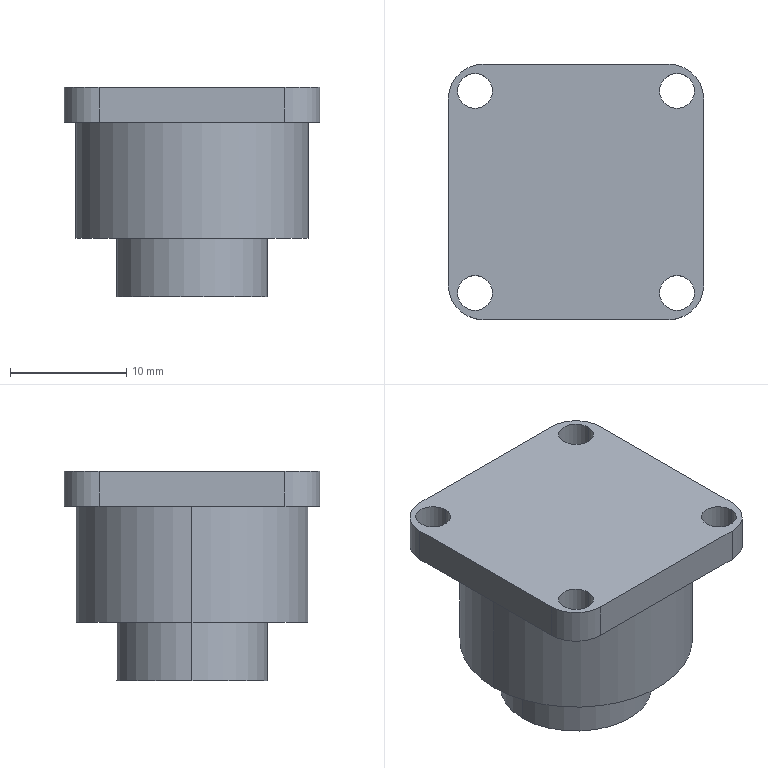Part | SolidWorks | features ICE 2, Cut 1, Extrusion 1, Fillet 1 | 1 solid | 27 faces | box 22 x 22 x 18 mm | volume 5008 mm3 | cylinder 18 | plane 9 | commonest cylinder face diameters 3 x8 6 x6 13 x2 20 x2
STEP:
#1=CARTESIAN_POINT('',(-155.946,-8.7,18.));
#2=VERTEX_POINT('',#1);
#3=CARTESIAN_POINT('',(-158.946,-8.7,18.));
#4=VERTEX_POINT('',#3);
#5=CARTESIAN_POINT('',(-157.446,-8.7,18.));
#6=DIRECTION('',(0.,0.,-1.));
#7=DIRECTION('',(-1.,0.,0.));
#8=AXIS2_PLACEMENT_3D('',#5,#6,#7);
#9=CIRCLE('',#8,1.5);
#10=EDGE_CURVE('',#2,#4,#9,.T.);
#11=ORIENTED_EDGE('',*,*,#10,.F.);
#12=CARTESIAN_POINT('',(-155.946,-8.7,15.));
#13=VERTEX_POINT('',#12);
#14=CARTESIAN_POINT('',(-155.946,-8.7,18.));
#15=DIRECTION('',(0.,0.,-1.));
#16=VECTOR('',#15,1000.);
#17=LINE('',#14,#16);
#18=EDGE_CURVE('',#2,#13,#17,.T.);
#19=ORIENTED_EDGE('',*,*,#18,.T.);
#20=CARTESIAN_POINT('',(-158.946,-8.7,15.));
#21=VERTEX_POINT('',#20);
#22=CARTESIAN_POINT('',(-157.446,-8.7,15.));
#23=DIRECTION('',(0.,0.,-1.));
#24=DIRECTION('',(-1.,0.,0.));
#25=AXIS2_PLACEMENT_3D('',#22,#23,#24);
#26=CIRCLE('',#25,1.5);
#27=EDGE_CURVE('',#13,#21,#26,.T.);
#28=ORIENTED_EDGE('',*,*,#27,.T.);
#29=CARTESIAN_POINT('',(-158.946,-8.7,18.));
#30=DIRECTION('',(0.,0.,-1.));
#31=VECTOR('',#30,1000.);
#32=LINE('',#29,#31);
#33=EDGE_CURVE('',#4,#21,#32,.T.);
#34=ORIENTED_EDGE('',*,*,#33,.F.);
#35=EDGE_LOOP('',(#11,#19,#28,#34));
#36=FACE_OUTER_BOUND('',#35,.T.);
#37=CARTESIAN_POINT('',(-157.446,-8.7,18.));
#38=DIRECTION('',(0.,0.,-1.));
#39=DIRECTION('',(-1.,0.,0.));
#40=AXIS2_PLACEMENT_3D('',#37,#38,#39);
#41=CYLINDRICAL_SURFACE('',#40,1.5);
#42=ADVANCED_FACE('',(#36),#41,.F.);
#43=CARTESIAN_POINT('',(-138.546,-8.7,18.));
#44=VERTEX_POINT('',#43);
#45=CARTESIAN_POINT('',(-141.546,-8.7,18.));
#46=VERTEX_POINT('',#45);
#47=CARTESIAN_POINT('',(-140.046,-8.7,18.));
#48=DIRECTION('',(0.,0.,-1.));
#49=DIRECTION('',(-1.,0.,0.));
#50=AXIS2_PLACEMENT_3D('',#47,#48,#49);
#51=CIRCLE('',#50,1.5);
#52=EDGE_CURVE('',#44,#46,#51,.T.);
#53=ORIENTED_EDGE('',*,*,#52,.F.);
#54=CARTESIAN_POINT('',(-138.546,-8.7,15.));
#55=VERTEX_POINT('',#54);
#56=CARTESIAN_POINT('',(-138.546,-8.7,18.));
#57=DIRECTION('',(0.,0.,-1.));
#58=VECTOR('',#57,1000.);
#59=LINE('',#56,#58);
#60=EDGE_CURVE('',#44,#55,#59,.T.);
#61=ORIENTED_EDGE('',*,*,#60,.T.);
#62=CARTESIAN_POINT('',(-141.546,-8.7,15.));
#63=VERTEX_POINT('',#62);
#64=CARTESIAN_POINT('',(-140.046,-8.7,15.));
#65=DIRECTION('',(0.,0.,-1.));
#66=DIRECTION('',(-1.,0.,0.));
#67=AXIS2_PLACEMENT_3D('',#64,#65,#66);
#68=CIRCLE('',#67,1.5);
#69=EDGE_CURVE('',#55,#63,#68,.T.);
#70=ORIENTED_EDGE('',*,*,#69,.T.);
#71=CARTESIAN_POINT('',(-141.546,-8.7,18.));
#72=DIRECTION('',(0.,0.,-1.));
#73=VECTOR('',#72,1000.);
#74=LINE('',#71,#73);
#75=EDGE_CURVE('',#46,#63,#74,.T.);
#76=ORIENTED_EDGE('',*,*,#75,.F.);
#77=EDGE_LOOP('',(#53,#61,#70,#76));
#78=FACE_OUTER_BOUND('',#77,.T.);
#79=CARTESIAN_POINT('',(-140.046,-8.7,18.));
#80=DIRECTION('',(0.,0.,-1.));
#81=DIRECTION('',(-1.,0.,0.));
#82=AXIS2_PLACEMENT_3D('',#79,#80,#81);
#83=CYLINDRICAL_SURFACE('',#82,1.5);
#84=ADVANCED_FACE('',(#78),#83,.F.);
#85=CARTESIAN_POINT('',(-138.546,8.7,18.));
#86=VERTEX_POINT('',#85);
#87=CARTESIAN_POINT('',(-141.546,8.7,18.));
#88=VERTEX_POINT('',#87);
#89=CARTESIAN_POINT('',(-140.046,8.7,18.));
#90=DIRECTION('',(0.,0.,-1.));
#91=DIRECTION('',(-1.,0.,0.));
#92=AXIS2_PLACEMENT_3D('',#89,#90,#91);
#93=CIRCLE('',#92,1.5);
#94=EDGE_CURVE('',#86,#88,#93,.T.);
#95=ORIENTED_EDGE('',*,*,#94,.F.);
#96=CARTESIAN_POINT('',(-138.546,8.7,15.));
#97=VERTEX_POINT('',#96);
#98=CARTESIAN_POINT('',(-138.546,8.7,18.));
#99=DIRECTION('',(0.,0.,-1.));
#100=VECTOR('',#99,1000.);
#101=LINE('',#98,#100);
#102=EDGE_CURVE('',#86,#97,#101,.T.);
#103=ORIENTED_EDGE('',*,*,#102,.T.);
#104=CARTESIAN_POINT('',(-141.546,8.7,15.));
#105=VERTEX_POINT('',#104);
#106=CARTESIAN_POINT('',(-140.046,8.7,15.));
#107=DIRECTION('',(0.,0.,-1.));
#108=DIRECTION('',(-1.,0.,0.));
#109=AXIS2_PLACEMENT_3D('',#106,#107,#108);
#110=CIRCLE('',#109,1.5);
#111=EDGE_CURVE('',#97,#105,#110,.T.);
#112=ORIENTED_EDGE('',*,*,#111,.T.);
#113=CARTESIAN_POINT('',(-141.546,8.7,18.));
#114=DIRECTION('',(0.,0.,-1.));
#115=VECTOR('',#114,1000.);
#116=LINE('',#113,#115);
#117=EDGE_CURVE('',#88,#105,#116,.T.);
#118=ORIENTED_EDGE('',*,*,#117,.F.);
#119=EDGE_LOOP('',(#95,#103,#112,#118));
#120=FACE_OUTER_BOUND('',#119,.T.);
#121=CARTESIAN_POINT('',(-140.046,8.7,18.));
#122=DIRECTION('',(0.,0.,-1.));
#123=DIRECTION('',(-1.,0.,0.));
#124=AXIS2_PLACEMENT_3D('',#121,#122,#123);
#125=CYLINDRICAL_SURFACE('',#124,1.5);
#126=ADVANCED_FACE('',(#120),#125,.F.);
#127=CARTESIAN_POINT('',(-155.946,8.7,18.));
#128=VERTEX_POINT('',#127);
#129=CARTESIAN_POINT('',(-158.946,8.7,18.));
#130=VERTEX_POINT('',#129);
#131=CARTESIAN_POINT('',(-157.446,8.7,18.));
#132=DIRECTION('',(0.,0.,-1.));
#133=DIRECTION('',(-1.,0.,0.));
#134=AXIS2_PLACEMENT_3D('',#131,#132,#133);
#135=CIRCLE('',#134,1.5);
#136=EDGE_CURVE('',#128,#130,#135,.T.);
#137=ORIENTED_EDGE('',*,*,#136,.F.);
#138=CARTESIAN_POINT('',(-155.946,8.7,15.));
#139=VERTEX_POINT('',#138);
#140=CARTESIAN_POINT('',(-155.946,8.7,18.));
#141=DIRECTION('',(0.,0.,-1.));
#142=VECTOR('',#141,1000.);
#143=LINE('',#140,#142);
#144=EDGE_CURVE('',#128,#139,#143,.T.);
#145=ORIENTED_EDGE('',*,*,#144,.T.);
#146=CARTESIAN_POINT('',(-158.946,8.7,15.));
#147=VERTEX_POINT('',#146);
#148=CARTESIAN_POINT('',(-157.446,8.7,15.));
#149=DIRECTION('',(0.,0.,-1.));
#150=DIRECTION('',(-1.,0.,0.));
#151=AXIS2_PLACEMENT_3D('',#148,#149,#150);
#152=CIRCLE('',#151,1.5);
#153=EDGE_CURVE('',#139,#147,#152,.T.);
#154=ORIENTED_EDGE('',*,*,#153,.T.);
#155=CARTESIAN_POINT('',(-158.946,8.7,18.));
#156=DIRECTION('',(0.,0.,-1.));
#157=VECTOR('',#156,1000.);
#158=LINE('',#155,#157);
#159=EDGE_CURVE('',#130,#147,#158,.T.);
#160=ORIENTED_EDGE('',*,*,#159,.F.);
#161=EDGE_LOOP('',(#137,#145,#154,#160));
#162=FACE_OUTER_BOUND('',#161,.T.);
#163=CARTESIAN_POINT('',(-157.446,8.7,18.));
#164=DIRECTION('',(0.,0.,-1.));
#165=DIRECTION('',(-1.,0.,0.));
#166=AXIS2_PLACEMENT_3D('',#163,#164,#165);
#167=CYLINDRICAL_SURFACE('',#166,1.5);
#168=ADVANCED_FACE('',(#162),#167,.F.);
#169=CARTESIAN_POINT('',(-138.746,0.,15.));
#170=VERTEX_POINT('',#169);
#171=CARTESIAN_POINT('',(-158.746,0.,15.));
#172=VERTEX_POINT('',#171);
#173=CARTESIAN_POINT('',(-148.746,0.,15.));
#174=DIRECTION('',(0.,0.,1.));
#175=DIRECTION('',(1.,0.,0.));
#176=AXIS2_PLACEMENT_3D('',#173,#174,#175);
#177=CIRCLE('',#176,10.);
#178=EDGE_CURVE('',#170,#172,#177,.T.);
#179=ORIENTED_EDGE('',*,*,#178,.F.);
#180=CARTESIAN_POINT('',(-138.746,0.,5.));
#181=VERTEX_POINT('',#180);
#182=CARTESIAN_POINT('',(-138.746,0.,15.));
#183=DIRECTION('',(0.,0.,-1.));
#184=VECTOR('',#183,1000.);
#185=LINE('',#182,#184);
#186=EDGE_CURVE('',#170,#181,#185,.T.);
#187=ORIENTED_EDGE('',*,*,#186,.T.);
#188=CARTESIAN_POINT('',(-158.746,0.,5.));
#189=VERTEX_POINT('',#188);
#190=CARTESIAN_POINT('',(-148.746,0.,5.));
#191=DIRECTION('',(0.,0.,1.));
#192=DIRECTION('',(1.,0.,0.));
#193=AXIS2_PLACEMENT_3D('',#190,#191,#192);
#194=CIRCLE('',#193,10.);
#195=EDGE_CURVE('',#181,#189,#194,.T.);
#196=ORIENTED_EDGE('',*,*,#195,.T.);
#197=CARTESIAN_POINT('',(-158.746,0.,15.));
#198=DIRECTION('',(0.,0.,-1.));
#199=VECTOR('',#198,1000.);
#200=LINE('',#197,#199);
#201=EDGE_CURVE('',#172,#189,#200,.T.);
#202=ORIENTED_EDGE('',*,*,#201,.F.);
#203=EDGE_LOOP('',(#179,#187,#196,#202));
#204=FACE_OUTER_BOUND('',#203,.T.);
#205=CARTESIAN_POINT('',(-148.746,0.,15.));
#206=DIRECTION('',(0.,0.,-1.));
#207=DIRECTION('',(-1.,0.,0.));
#208=AXIS2_PLACEMENT_3D('',#205,#206,#207);
#209=CYLINDRICAL_SURFACE('',#208,10.);
#210=ADVANCED_FACE('',(#204),#209,.T.);
#211=CARTESIAN_POINT('',(-151.746,0.,5.));
#212=VERTEX_POINT('',#211);
#213=CARTESIAN_POINT('',(-145.746,0.,5.));
#214=VERTEX_POINT('',#213);
#215=CARTESIAN_POINT('',(-148.746,0.,5.));
#216=DIRECTION('',(0.,0.,1.));
#217=DIRECTION('',(1.,0.,0.));
#218=AXIS2_PLACEMENT_3D('',#215,#216,#217);
#219=CIRCLE('',#218,3.);
#220=EDGE_CURVE('',#212,#214,#219,.T.);
#221=ORIENTED_EDGE('',*,*,#220,.T.);
#222=CARTESIAN_POINT('',(-145.746,0.,0.));
#223=VERTEX_POINT('',#222);
#224=CARTESIAN_POINT('',(-145.746,0.,5.));
#225=DIRECTION('',(0.,0.,-1.));
#226=VECTOR('',#225,1000.);
#227=LINE('',#224,#226);
#228=EDGE_CURVE('',#214,#223,#227,.T.);
#229=ORIENTED_EDGE('',*,*,#228,.T.);
#230=CARTESIAN_POINT('',(-151.746,0.,0.));
#231=VERTEX_POINT('',#230);
#232=CARTESIAN_POINT('',(-148.746,0.,0.));
#233=DIRECTION('',(0.,0.,1.));
#234=DIRECTION('',(1.,0.,0.));
#235=AXIS2_PLACEMENT_3D('',#232,#233,#234);
#236=CIRCLE('',#235,3.);
#237=EDGE_CURVE('',#231,#223,#236,.T.);
#238=ORIENTED_EDGE('',*,*,#237,.F.);
#239=CARTESIAN_POINT('',(-151.746,0.,5.));
#240=DIRECTION('',(0.,0.,-1.));
#241=VECTOR('',#240,1000.);
#242=LINE('',#239,#241);
#243=EDGE_CURVE('',#212,#231,#242,.T.);
#244=ORIENTED_EDGE('',*,*,#243,.F.);
#245=EDGE_LOOP('',(#221,#229,#238,#244));
#246=FACE_OUTER_BOUND('',#245,.T.);
#247=CARTESIAN_POINT('',(-148.746,0.,5.));
#248=DIRECTION('',(0.,0.,-1.));
#249=DIRECTION('',(-1.,0.,0.));
#250=AXIS2_PLACEMENT_3D('',#247,#248,#249);
#251=CYLINDRICAL_SURFACE('',#250,3.);
#252=ADVANCED_FACE('',(#246),#251,.F.);
#253=CARTESIAN_POINT('',(-142.246,0.,5.));
#254=VERTEX_POINT('',#253);
#255=CARTESIAN_POINT('',(-155.246,0.,5.));
#256=VERTEX_POINT('',#255);
#257=CARTESIAN_POINT('',(-148.746,0.,5.));
#258=DIRECTION('',(0.,0.,1.));
#259=DIRECTION('',(1.,0.,0.));
#260=AXIS2_PLACEMENT_3D('',#257,#258,#259);
#261=CIRCLE('',#260,6.5);
#262=EDGE_CURVE('',#254,#256,#261,.T.);
#263=ORIENTED_EDGE('',*,*,#262,.F.);
#264=CARTESIAN_POINT('',(-142.246,0.,0.));
#265=VERTEX_POINT('',#264);
#266=CARTESIAN_POINT('',(-142.246,0.,5.));
#267=DIRECTION('',(0.,0.,-1.));
#268=VECTOR('',#267,1000.);
#269=LINE('',#266,#268);
#270=EDGE_CURVE('',#254,#265,#269,.T.);
#271=ORIENTED_EDGE('',*,*,#270,.T.);
#272=CARTESIAN_POINT('',(-155.246,0.,0.));
#273=VERTEX_POINT('',#272);
#274=CARTESIAN_POINT('',(-148.746,0.,0.));
#275=DIRECTION('',(0.,0.,1.));
#276=DIRECTION('',(1.,0.,0.));
#277=AXIS2_PLACEMENT_3D('',#274,#275,#276);
#278=CIRCLE('',#277,6.5);
#279=EDGE_CURVE('',#265,#273,#278,.T.);
#280=ORIENTED_EDGE('',*,*,#279,.T.);
#281=CARTESIAN_POINT('',(-155.246,0.,5.));
#282=DIRECTION('',(0.,0.,-1.));
#283=VECTOR('',#282,1000.);
#284=LINE('',#281,#283);
#285=EDGE_CURVE('',#256,#273,#284,.T.);
#286=ORIENTED_EDGE('',*,*,#285,.F.);
#287=EDGE_LOOP('',(#263,#271,#280,#286));
#288=FACE_OUTER_BOUND('',#287,.T.);
#289=CARTESIAN_POINT('',(-148.746,0.,5.));
#290=DIRECTION('',(0.,0.,-1.));
#291=DIRECTION('',(-1.,0.,0.));
#292=AXIS2_PLACEMENT_3D('',#289,#290,#291);
#293=CYLINDRICAL_SURFACE('',#292,6.5);
#294=ADVANCED_FACE('',(#288),#293,.T.);
#295=CARTESIAN_POINT('',(-148.746,0.,0.));
#296=DIRECTION('',(0.,0.,1.));
#297=DIRECTION('',(1.,0.,0.));
#298=AXIS2_PLACEMENT_3D('',#295,#296,#297);
#299=CIRCLE('',#298,6.5);
#300=EDGE_CURVE('',#273,#265,#299,.T.);
#301=ORIENTED_EDGE('',*,*,#300,.F.);
#302=ORIENTED_EDGE('',*,*,#279,.F.);
#303=EDGE_LOOP('',(#301,#302));
#304=FACE_OUTER_BOUND('',#303,.T.);
#305=ORIENTED_EDGE('',*,*,#237,.T.);
#306=CARTESIAN_POINT('',(-148.746,0.,0.));
#307=DIRECTION('',(0.,0.,1.));
#308=DIRECTION('',(1.,0.,0.));
#309=AXIS2_PLACEMENT_3D('',#306,#307,#308);
#310=CIRCLE('',#309,3.);
#311=EDGE_CURVE('',#223,#231,#310,.T.);
#312=ORIENTED_EDGE('',*,*,#311,.T.);
#313=EDGE_LOOP('',(#305,#312));
#314=FACE_BOUND('',#313,.T.);
#315=CARTESIAN_POINT('',(-148.746,0.,0.));
#316=DIRECTION('',(0.,0.,1.));
#317=DIRECTION('',(1.,0.,0.));
#318=AXIS2_PLACEMENT_3D('',#315,#316,#317);
#319=PLANE('',#318);
#320=ADVANCED_FACE('',(#304,#314),#319,.F.);
#321=ORIENTED_EDGE('',*,*,#270,.F.);
#322=CARTESIAN_POINT('',(-148.746,0.,5.));
#323=DIRECTION('',(0.,0.,1.));
#324=DIRECTION('',(1.,0.,0.));
#325=AXIS2_PLACEMENT_3D('',#322,#323,#324);
#326=CIRCLE('',#325,6.5);
#327=EDGE_CURVE('',#256,#254,#326,.T.);
#328=ORIENTED_EDGE('',*,*,#327,.F.);
#329=ORIENTED_EDGE('',*,*,#285,.T.);
#330=ORIENTED_EDGE('',*,*,#300,.T.);
#331=EDGE_LOOP('',(#321,#328,#329,#330));
#332=FACE_OUTER_BOUND('',#331,.T.);
#333=CARTESIAN_POINT('',(-148.746,0.,5.));
#334=DIRECTION('',(0.,0.,-1.));
#335=DIRECTION('',(-1.,0.,0.));
#336=AXIS2_PLACEMENT_3D('',#333,#334,#335);
#337=CYLINDRICAL_SURFACE('',#336,6.5);
#338=ADVANCED_FACE('',(#332),#337,.T.);
#339=ORIENTED_EDGE('',*,*,#228,.F.);
#340=CARTESIAN_POINT('',(-148.746,0.,5.));
#341=DIRECTION('',(0.,0.,1.));
#342=DIRECTION('',(1.,0.,0.));
#343=AXIS2_PLACEMENT_3D('',#340,#341,#342);
#344=CIRCLE('',#343,3.);
#345=EDGE_CURVE('',#214,#212,#344,.T.);
#346=ORIENTED_EDGE('',*,*,#345,.T.);
#347=ORIENTED_EDGE('',*,*,#243,.T.);
#348=ORIENTED_EDGE('',*,*,#311,.F.);
#349=EDGE_LOOP('',(#339,#346,#347,#348));
#350=FACE_OUTER_BOUND('',#349,.T.);
#351=CARTESIAN_POINT('',(-148.746,0.,5.));
#352=DIRECTION('',(0.,0.,-1.));
#353=DIRECTION('',(-1.,0.,0.));
#354=AXIS2_PLACEMENT_3D('',#351,#352,#353);
#355=CYLINDRICAL_SURFACE('',#354,3.);
#356=ADVANCED_FACE('',(#350),#355,.F.);
#357=ORIENTED_EDGE('',*,*,#220,.F.);
#358=ORIENTED_EDGE('',*,*,#345,.F.);
#359=EDGE_LOOP('',(#357,#358));
#360=FACE_OUTER_BOUND('',#359,.T.);
#361=CARTESIAN_POINT('',(-148.746,0.,5.));
#362=DIRECTION('',(0.,0.,1.));
#363=DIRECTION('',(1.,0.,0.));
#364=AXIS2_PLACEMENT_3D('',#361,#362,#363);
#365=PLANE('',#364);
#366=ADVANCED_FACE('',(#360),#365,.F.);
#367=ORIENTED_EDGE('',*,*,#186,.F.);
#368=CARTESIAN_POINT('',(-148.746,0.,15.));
#369=DIRECTION('',(0.,0.,1.));
#370=DIRECTION('',(1.,0.,0.));
#371=AXIS2_PLACEMENT_3D('',#368,#369,#370);
#372=CIRCLE('',#371,10.);
#373=EDGE_CURVE('',#172,#170,#372,.T.);
#374=ORIENTED_EDGE('',*,*,#373,.F.);
#375=ORIENTED_EDGE('',*,*,#201,.T.);
#376=CARTESIAN_POINT('',(-148.746,0.,5.));
#377=DIRECTION('',(0.,0.,1.));
#378=DIRECTION('',(1.,0.,0.));
#379=AXIS2_PLACEMENT_3D('',#376,#377,#378);
#380=CIRCLE('',#379,10.);
#381=EDGE_CURVE('',#189,#181,#380,.T.);
#382=ORIENTED_EDGE('',*,*,#381,.T.);
#383=EDGE_LOOP('',(#367,#374,#375,#382));
#384=FACE_OUTER_BOUND('',#383,.T.);
#385=CARTESIAN_POINT('',(-148.746,0.,15.));
#386=DIRECTION('',(0.,0.,-1.));
#387=DIRECTION('',(-1.,0.,0.));
#388=AXIS2_PLACEMENT_3D('',#385,#386,#387);
#389=CYLINDRICAL_SURFACE('',#388,10.);
#390=ADVANCED_FACE('',(#384),#389,.T.);
#391=ORIENTED_EDGE('',*,*,#327,.T.);
#392=ORIENTED_EDGE('',*,*,#262,.T.);
#393=EDGE_LOOP('',(#391,#392));
#394=FACE_BOUND('',#393,.T.);
#395=ORIENTED_EDGE('',*,*,#381,.F.);
#396=ORIENTED_EDGE('',*,*,#195,.F.);
#397=EDGE_LOOP('',(#395,#396));
#398=FACE_OUTER_BOUND('',#397,.T.);
#399=CARTESIAN_POINT('',(-148.746,0.,5.));
#400=DIRECTION('',(0.,0.,1.));
#401=DIRECTION('',(1.,0.,0.));
#402=AXIS2_PLACEMENT_3D('',#399,#400,#401);
#403=PLANE('',#402);
#404=ADVANCED_FACE('',(#394,#398),#403,.F.);
#405=CARTESIAN_POINT('',(-137.746,-8.,15.));
#406=VERTEX_POINT('',#405);
#407=CARTESIAN_POINT('',(-137.746,8.,15.));
#408=VERTEX_POINT('',#407);
#409=CARTESIAN_POINT('',(-137.746,-11.,15.));
#410=DIRECTION('',(0.,1.,0.));
#411=VECTOR('',#410,1000.);
#412=LINE('',#409,#411);
#413=EDGE_CURVE('',#406,#408,#412,.T.);
#414=ORIENTED_EDGE('',*,*,#413,.T.);
#415=CARTESIAN_POINT('',(-137.746,8.,18.));
#416=VERTEX_POINT('',#415);
#417=CARTESIAN_POINT('',(-137.746,8.,18.));
#418=DIRECTION('',(0.,0.,1.));
#419=VECTOR('',#418,1000.);
#420=LINE('',#417,#419);
#421=EDGE_CURVE('',#408,#416,#420,.T.);
#422=ORIENTED_EDGE('',*,*,#421,.T.);
#423=CARTESIAN_POINT('',(-137.746,-8.,18.));
#424=VERTEX_POINT('',#423);
#425=CARTESIAN_POINT('',(-137.746,-11.,18.));
#426=DIRECTION('',(0.,1.,0.));
#427=VECTOR('',#426,1000.);
#428=LINE('',#425,#427);
#429=EDGE_CURVE('',#424,#416,#428,.T.);
#430=ORIENTED_EDGE('',*,*,#429,.F.);
#431=CARTESIAN_POINT('',(-137.746,-8.,18.));
#432=DIRECTION('',(0.,0.,-1.));
#433=VECTOR('',#432,1000.);
#434=LINE('',#431,#433);
#435=EDGE_CURVE('',#424,#406,#434,.T.);
#436=ORIENTED_EDGE('',*,*,#435,.T.);
#437=EDGE_LOOP('',(#414,#422,#430,#436));
#438=FACE_OUTER_BOUND('',#437,.T.);
#439=CARTESIAN_POINT('',(-137.746,-11.,18.));
#440=DIRECTION('',(-1.,0.,0.));
#441=DIRECTION('',(0.,0.,1.));
#442=AXIS2_PLACEMENT_3D('',#439,#440,#441);
#443=PLANE('',#442);
#444=ADVANCED_FACE('',(#438),#443,.F.);
#445=CARTESIAN_POINT('',(-140.746,11.,18.));
#446=VERTEX_POINT('',#445);
#447=CARTESIAN_POINT('',(-156.746,11.,18.));
#448=VERTEX_POINT('',#447);
#449=CARTESIAN_POINT('',(-159.746,11.,18.));
#450=DIRECTION('',(-1.,0.,0.));
#451=VECTOR('',#450,1000.);
#452=LINE('',#449,#451);
#453=EDGE_CURVE('',#446,#448,#452,.T.);
#454=ORIENTED_EDGE('',*,*,#453,.F.);
#455=CARTESIAN_POINT('',(-140.746,11.,15.));
#456=VERTEX_POINT('',#455);
#457=CARTESIAN_POINT('',(-140.746,11.,18.));
#458=DIRECTION('',(0.,0.,-1.));
#459=VECTOR('',#458,1000.);
#460=LINE('',#457,#459);
#461=EDGE_CURVE('',#446,#456,#460,.T.);
#462=ORIENTED_EDGE('',*,*,#461,.T.);
#463=CARTESIAN_POINT('',(-156.746,11.,15.));
#464=VERTEX_POINT('',#463);
#465=CARTESIAN_POINT('',(-159.746,11.,15.));
#466=DIRECTION('',(-1.,0.,0.));
#467=VECTOR('',#466,1000.);
#468=LINE('',#465,#467);
#469=EDGE_CURVE('',#456,#464,#468,.T.);
#470=ORIENTED_EDGE('',*,*,#469,.T.);
#471=CARTESIAN_POINT('',(-156.746,11.,18.));
#472=DIRECTION('',(0.,0.,1.));
#473=VECTOR('',#472,1000.);
#474=LINE('',#471,#473);
#475=EDGE_CURVE('',#464,#448,#474,.T.);
#476=ORIENTED_EDGE('',*,*,#475,.T.);
#477=EDGE_LOOP('',(#454,#462,#470,#476));
#478=FACE_OUTER_BOUND('',#477,.T.);
#479=CARTESIAN_POINT('',(-159.746,11.,18.));
#480=DIRECTION('',(0.,-1.,0.));
#481=DIRECTION('',(0.,0.,-1.));
#482=AXIS2_PLACEMENT_3D('',#479,#480,#481);
#483=PLANE('',#482);
#484=ADVANCED_FACE('',(#478),#483,.F.);
#485=CARTESIAN_POINT('',(-159.746,8.,15.));
#486=VERTEX_POINT('',#485);
#487=CARTESIAN_POINT('',(-159.746,-8.,15.));
#488=VERTEX_POINT('',#487);
#489=CARTESIAN_POINT('',(-159.746,-11.,15.));
#490=DIRECTION('',(0.,-1.,0.));
#491=VECTOR('',#490,1000.);
#492=LINE('',#489,#491);
#493=EDGE_CURVE('',#486,#488,#492,.T.);
#494=ORIENTED_EDGE('',*,*,#493,.T.);
#495=CARTESIAN_POINT('',(-159.746,-8.,18.));
#496=VERTEX_POINT('',#495);
#497=CARTESIAN_POINT('',(-159.746,-8.,18.));
#498=DIRECTION('',(0.,0.,1.));
#499=VECTOR('',#498,1000.);
#500=LINE('',#497,#499);
#501=EDGE_CURVE('',#488,#496,#500,.T.);
#502=ORIENTED_EDGE('',*,*,#501,.T.);
#503=CARTESIAN_POINT('',(-159.746,8.,18.));
#504=VERTEX_POINT('',#503);
#505=CARTESIAN_POINT('',(-159.746,-11.,18.));
#506=DIRECTION('',(0.,-1.,0.));
#507=VECTOR('',#506,1000.);
#508=LINE('',#505,#507);
#509=EDGE_CURVE('',#504,#496,#508,.T.);
#510=ORIENTED_EDGE('',*,*,#509,.F.);
#511=CARTESIAN_POINT('',(-159.746,8.,18.));
#512=DIRECTION('',(0.,0.,-1.));
#513=VECTOR('',#512,1000.);
#514=LINE('',#511,#513);
#515=EDGE_CURVE('',#504,#486,#514,.T.);
#516=ORIENTED_EDGE('',*,*,#515,.T.);
#517=EDGE_LOOP('',(#494,#502,#510,#516));
#518=FACE_OUTER_BOUND('',#517,.T.);
#519=CARTESIAN_POINT('',(-159.746,-11.,18.));
#520=DIRECTION('',(1.,0.,0.));
#521=DIRECTION('',(0.,0.,-1.));
#522=AXIS2_PLACEMENT_3D('',#519,#520,#521);
#523=PLANE('',#522);
#524=ADVANCED_FACE('',(#518),#523,.F.);
#525=CARTESIAN_POINT('',(-156.746,-11.,18.));
#526=VERTEX_POINT('',#525);
#527=CARTESIAN_POINT('',(-140.746,-11.,18.));
#528=VERTEX_POINT('',#527);
#529=CARTESIAN_POINT('',(-159.746,-11.,18.));
#530=DIRECTION('',(1.,0.,0.));
#531=VECTOR('',#530,1000.);
#532=LINE('',#529,#531);
#533=EDGE_CURVE('',#526,#528,#532,.T.);
#534=ORIENTED_EDGE('',*,*,#533,.F.);
#535=CARTESIAN_POINT('',(-156.746,-11.,15.));
#536=VERTEX_POINT('',#535);
#537=CARTESIAN_POINT('',(-156.746,-11.,18.));
#538=DIRECTION('',(0.,0.,-1.));
#539=VECTOR('',#538,1000.);
#540=LINE('',#537,#539);
#541=EDGE_CURVE('',#526,#536,#540,.T.);
#542=ORIENTED_EDGE('',*,*,#541,.T.);
#543=CARTESIAN_POINT('',(-140.746,-11.,15.));
#544=VERTEX_POINT('',#543);
#545=CARTESIAN_POINT('',(-159.746,-11.,15.));
#546=DIRECTION('',(1.,0.,0.));
#547=VECTOR('',#546,1000.);
#548=LINE('',#545,#547);
#549=EDGE_CURVE('',#536,#544,#548,.T.);
#550=ORIENTED_EDGE('',*,*,#549,.T.);
#551=CARTESIAN_POINT('',(-140.746,-11.,18.));
#552=DIRECTION('',(0.,0.,1.));
#553=VECTOR('',#552,1000.);
#554=LINE('',#551,#553);
#555=EDGE_CURVE('',#544,#528,#554,.T.);
#556=ORIENTED_EDGE('',*,*,#555,.T.);
#557=EDGE_LOOP('',(#534,#542,#550,#556));
#558=FACE_OUTER_BOUND('',#557,.T.);
#559=CARTESIAN_POINT('',(-159.746,-11.,18.));
#560=DIRECTION('',(0.,1.,0.));
#561=DIRECTION('',(0.,0.,1.));
#562=AXIS2_PLACEMENT_3D('',#559,#560,#561);
#563=PLANE('',#562);
#564=ADVANCED_FACE('',(#558),#563,.F.);
#565=CARTESIAN_POINT('',(-157.446,-8.7,18.));
#566=DIRECTION('',(0.,0.,-1.));
#567=DIRECTION('',(-1.,0.,0.));
#568=AXIS2_PLACEMENT_3D('',#565,#566,#567);
#569=CIRCLE('',#568,1.5);
#570=EDGE_CURVE('',#4,#2,#569,.T.);
#571=ORIENTED_EDGE('',*,*,#570,.T.);
#572=ORIENTED_EDGE('',*,*,#10,.T.);
#573=EDGE_LOOP('',(#571,#572));
#574=FACE_BOUND('',#573,.T.);
#575=CARTESIAN_POINT('',(-140.046,-8.7,18.));
#576=DIRECTION('',(0.,0.,-1.));
#577=DIRECTION('',(-1.,0.,0.));
#578=AXIS2_PLACEMENT_3D('',#575,#576,#577);
#579=CIRCLE('',#578,1.5);
#580=EDGE_CURVE('',#46,#44,#579,.T.);
#581=ORIENTED_EDGE('',*,*,#580,.T.);
#582=ORIENTED_EDGE('',*,*,#52,.T.);
#583=EDGE_LOOP('',(#581,#582));
#584=FACE_BOUND('',#583,.T.);
#585=CARTESIAN_POINT('',(-140.046,8.7,18.));
#586=DIRECTION('',(0.,0.,-1.));
#587=DIRECTION('',(-1.,0.,0.));
#588=AXIS2_PLACEMENT_3D('',#585,#586,#587);
#589=CIRCLE('',#588,1.5);
#590=EDGE_CURVE('',#88,#86,#589,.T.);
#591=ORIENTED_EDGE('',*,*,#590,.T.);
#592=ORIENTED_EDGE('',*,*,#94,.T.);
#593=EDGE_LOOP('',(#591,#592));
#594=FACE_BOUND('',#593,.T.);
#595=CARTESIAN_POINT('',(-157.446,8.7,18.));
#596=DIRECTION('',(0.,0.,-1.));
#597=DIRECTION('',(-1.,0.,0.));
#598=AXIS2_PLACEMENT_3D('',#595,#596,#597);
#599=CIRCLE('',#598,1.5);
#600=EDGE_CURVE('',#130,#128,#599,.T.);
#601=ORIENTED_EDGE('',*,*,#600,.T.);
#602=ORIENTED_EDGE('',*,*,#136,.T.);
#603=EDGE_LOOP('',(#601,#602));
#604=FACE_BOUND('',#603,.T.);
#605=ORIENTED_EDGE('',*,*,#429,.T.);
#606=CARTESIAN_POINT('',(-140.746,8.,18.));
#607=DIRECTION('',(0.,0.,1.));
#608=DIRECTION('',(-1.,0.,0.));
#609=AXIS2_PLACEMENT_3D('',#606,#607,#608);
#610=CIRCLE('',#609,3.);
#611=EDGE_CURVE('',#416,#446,#610,.T.);
#612=ORIENTED_EDGE('',*,*,#611,.T.);
#613=ORIENTED_EDGE('',*,*,#453,.T.);
#614=CARTESIAN_POINT('',(-156.746,8.,18.));
#615=DIRECTION('',(0.,0.,1.));
#616=DIRECTION('',(-1.,0.,0.));
#617=AXIS2_PLACEMENT_3D('',#614,#615,#616);
#618=CIRCLE('',#617,3.);
#619=EDGE_CURVE('',#448,#504,#618,.T.);
#620=ORIENTED_EDGE('',*,*,#619,.T.);
#621=ORIENTED_EDGE('',*,*,#509,.T.);
#622=CARTESIAN_POINT('',(-156.746,-8.,18.));
#623=DIRECTION('',(0.,0.,1.));
#624=DIRECTION('',(-1.,0.,0.));
#625=AXIS2_PLACEMENT_3D('',#622,#623,#624);
#626=CIRCLE('',#625,3.);
#627=EDGE_CURVE('',#496,#526,#626,.T.);
#628=ORIENTED_EDGE('',*,*,#627,.T.);
#629=ORIENTED_EDGE('',*,*,#533,.T.);
#630=CARTESIAN_POINT('',(-140.746,-8.,18.));
#631=DIRECTION('',(0.,0.,1.));
#632=DIRECTION('',(-1.,0.,0.));
#633=AXIS2_PLACEMENT_3D('',#630,#631,#632);
#634=CIRCLE('',#633,3.);
#635=EDGE_CURVE('',#528,#424,#634,.T.);
#636=ORIENTED_EDGE('',*,*,#635,.T.);
#637=EDGE_LOOP('',(#605,#612,#613,#620,#621,#628,#629,#636));
#638=FACE_OUTER_BOUND('',#637,.T.);
#639=CARTESIAN_POINT('',(0.,0.,18.));
#640=DIRECTION('',(0.,0.,-1.));
#641=DIRECTION('',(-1.,0.,0.));
#642=AXIS2_PLACEMENT_3D('',#639,#640,#641);
#643=PLANE('',#642);
#644=ADVANCED_FACE('',(#574,#584,#594,#604,#638),#643,.F.);
#645=CARTESIAN_POINT('',(-157.446,-8.7,15.));
#646=DIRECTION('',(0.,0.,-1.));
#647=DIRECTION('',(-1.,0.,0.));
#648=AXIS2_PLACEMENT_3D('',#645,#646,#647);
#649=CIRCLE('',#648,1.5);
#650=EDGE_CURVE('',#21,#13,#649,.T.);
#651=ORIENTED_EDGE('',*,*,#650,.F.);
#652=ORIENTED_EDGE('',*,*,#27,.F.);
#653=EDGE_LOOP('',(#651,#652));
#654=FACE_BOUND('',#653,.T.);
#655=CARTESIAN_POINT('',(-140.046,-8.7,15.));
#656=DIRECTION('',(0.,0.,-1.));
#657=DIRECTION('',(-1.,0.,0.));
#658=AXIS2_PLACEMENT_3D('',#655,#656,#657);
#659=CIRCLE('',#658,1.5);
#660=EDGE_CURVE('',#63,#55,#659,.T.);
#661=ORIENTED_EDGE('',*,*,#660,.F.);
#662=ORIENTED_EDGE('',*,*,#69,.F.);
#663=EDGE_LOOP('',(#661,#662));
#664=FACE_BOUND('',#663,.T.);
#665=CARTESIAN_POINT('',(-140.046,8.7,15.));
#666=DIRECTION('',(0.,0.,-1.));
#667=DIRECTION('',(-1.,0.,0.));
#668=AXIS2_PLACEMENT_3D('',#665,#666,#667);
#669=CIRCLE('',#668,1.5);
#670=EDGE_CURVE('',#105,#97,#669,.T.);
#671=ORIENTED_EDGE('',*,*,#670,.F.);
#672=ORIENTED_EDGE('',*,*,#111,.F.);
#673=EDGE_LOOP('',(#671,#672));
#674=FACE_BOUND('',#673,.T.);
#675=CARTESIAN_POINT('',(-157.446,8.7,15.));
#676=DIRECTION('',(0.,0.,-1.));
#677=DIRECTION('',(-1.,0.,0.));
#678=AXIS2_PLACEMENT_3D('',#675,#676,#677);
#679=CIRCLE('',#678,1.5);
#680=EDGE_CURVE('',#147,#139,#679,.T.);
#681=ORIENTED_EDGE('',*,*,#680,.F.);
#682=ORIENTED_EDGE('',*,*,#153,.F.);
#683=EDGE_LOOP('',(#681,#682));
#684=FACE_BOUND('',#683,.T.);
#685=ORIENTED_EDGE('',*,*,#373,.T.);
#686=ORIENTED_EDGE('',*,*,#178,.T.);
#687=EDGE_LOOP('',(#685,#686));
#688=FACE_BOUND('',#687,.T.);
#689=ORIENTED_EDGE('',*,*,#469,.F.);
#690=CARTESIAN_POINT('',(-140.746,8.,15.));
#691=DIRECTION('',(0.,0.,-1.));
#692=DIRECTION('',(-1.,0.,0.));
#693=AXIS2_PLACEMENT_3D('',#690,#691,#692);
#694=CIRCLE('',#693,3.);
#695=EDGE_CURVE('',#456,#408,#694,.T.);
#696=ORIENTED_EDGE('',*,*,#695,.T.);
#697=ORIENTED_EDGE('',*,*,#413,.F.);
#698=CARTESIAN_POINT('',(-140.746,-8.,15.));
#699=DIRECTION('',(0.,0.,-1.));
#700=DIRECTION('',(-1.,0.,0.));
#701=AXIS2_PLACEMENT_3D('',#698,#699,#700);
#702=CIRCLE('',#701,3.);
#703=EDGE_CURVE('',#406,#544,#702,.T.);
#704=ORIENTED_EDGE('',*,*,#703,.T.);
#705=ORIENTED_EDGE('',*,*,#549,.F.);
#706=CARTESIAN_POINT('',(-156.746,-8.,15.));
#707=DIRECTION('',(0.,0.,-1.));
#708=DIRECTION('',(-1.,0.,0.));
#709=AXIS2_PLACEMENT_3D('',#706,#707,#708);
#710=CIRCLE('',#709,3.);
#711=EDGE_CURVE('',#536,#488,#710,.T.);
#712=ORIENTED_EDGE('',*,*,#711,.T.);
#713=ORIENTED_EDGE('',*,*,#493,.F.);
#714=CARTESIAN_POINT('',(-156.746,8.,15.));
#715=DIRECTION('',(0.,0.,-1.));
#716=DIRECTION('',(-1.,0.,0.));
#717=AXIS2_PLACEMENT_3D('',#714,#715,#716);
#718=CIRCLE('',#717,3.);
#719=EDGE_CURVE('',#486,#464,#718,.T.);
#720=ORIENTED_EDGE('',*,*,#719,.T.);
#721=EDGE_LOOP('',(#689,#696,#697,#704,#705,#712,#713,#720));
#722=FACE_OUTER_BOUND('',#721,.T.);
#723=CARTESIAN_POINT('',(0.,0.,15.));
#724=DIRECTION('',(0.,0.,-1.));
#725=DIRECTION('',(-1.,0.,0.));
#726=AXIS2_PLACEMENT_3D('',#723,#724,#725);
#727=PLANE('',#726);
#728=ADVANCED_FACE('',(#654,#664,#674,#684,#688,#722),#727,.T.);
#729=ORIENTED_EDGE('',*,*,#611,.F.);
#730=ORIENTED_EDGE('',*,*,#421,.F.);
#731=ORIENTED_EDGE('',*,*,#695,.F.);
#732=ORIENTED_EDGE('',*,*,#461,.F.);
#733=EDGE_LOOP('',(#729,#730,#731,#732));
#734=FACE_OUTER_BOUND('',#733,.T.);
#735=CARTESIAN_POINT('',(-140.746,8.,18.));
#736=DIRECTION('',(0.,0.,-1.));
#737=DIRECTION('',(-1.,0.,0.));
#738=AXIS2_PLACEMENT_3D('',#735,#736,#737);
#739=CYLINDRICAL_SURFACE('',#738,3.);
#740=ADVANCED_FACE('',(#734),#739,.T.);
#741=ORIENTED_EDGE('',*,*,#627,.F.);
#742=ORIENTED_EDGE('',*,*,#501,.F.);
#743=ORIENTED_EDGE('',*,*,#711,.F.);
#744=ORIENTED_EDGE('',*,*,#541,.F.);
#745=EDGE_LOOP('',(#741,#742,#743,#744));
#746=FACE_OUTER_BOUND('',#745,.T.);
#747=CARTESIAN_POINT('',(-156.746,-8.,18.));
#748=DIRECTION('',(0.,0.,-1.));
#749=DIRECTION('',(-1.,0.,0.));
#750=AXIS2_PLACEMENT_3D('',#747,#748,#749);
#751=CYLINDRICAL_SURFACE('',#750,3.);
#752=ADVANCED_FACE('',(#746),#751,.T.);
#753=ORIENTED_EDGE('',*,*,#635,.F.);
#754=ORIENTED_EDGE('',*,*,#555,.F.);
#755=ORIENTED_EDGE('',*,*,#703,.F.);
#756=ORIENTED_EDGE('',*,*,#435,.F.);
#757=EDGE_LOOP('',(#753,#754,#755,#756));
#758=FACE_OUTER_BOUND('',#757,.T.);
#759=CARTESIAN_POINT('',(-140.746,-8.,18.));
#760=DIRECTION('',(0.,0.,-1.));
#761=DIRECTION('',(-1.,0.,0.));
#762=AXIS2_PLACEMENT_3D('',#759,#760,#761);
#763=CYLINDRICAL_SURFACE('',#762,3.);
#764=ADVANCED_FACE('',(#758),#763,.T.);
#765=ORIENTED_EDGE('',*,*,#619,.F.);
#766=ORIENTED_EDGE('',*,*,#475,.F.);
#767=ORIENTED_EDGE('',*,*,#719,.F.);
#768=ORIENTED_EDGE('',*,*,#515,.F.);
#769=EDGE_LOOP('',(#765,#766,#767,#768));
#770=FACE_OUTER_BOUND('',#769,.T.);
#771=CARTESIAN_POINT('',(-156.746,8.,18.));
#772=DIRECTION('',(0.,0.,-1.));
#773=DIRECTION('',(-1.,0.,0.));
#774=AXIS2_PLACEMENT_3D('',#771,#772,#773);
#775=CYLINDRICAL_SURFACE('',#774,3.);
#776=ADVANCED_FACE('',(#770),#775,.T.);
#777=ORIENTED_EDGE('',*,*,#144,.F.);
#778=ORIENTED_EDGE('',*,*,#600,.F.);
#779=ORIENTED_EDGE('',*,*,#159,.T.);
#780=ORIENTED_EDGE('',*,*,#680,.T.);
#781=EDGE_LOOP('',(#777,#778,#779,#780));
#782=FACE_OUTER_BOUND('',#781,.T.);
#783=CARTESIAN_POINT('',(-157.446,8.7,18.));
#784=DIRECTION('',(0.,0.,-1.));
#785=DIRECTION('',(-1.,0.,0.));
#786=AXIS2_PLACEMENT_3D('',#783,#784,#785);
#787=CYLINDRICAL_SURFACE('',#786,1.5);
#788=ADVANCED_FACE('',(#782),#787,.F.);
#789=ORIENTED_EDGE('',*,*,#102,.F.);
#790=ORIENTED_EDGE('',*,*,#590,.F.);
#791=ORIENTED_EDGE('',*,*,#117,.T.);
#792=ORIENTED_EDGE('',*,*,#670,.T.);
#793=EDGE_LOOP('',(#789,#790,#791,#792));
#794=FACE_OUTER_BOUND('',#793,.T.);
#795=CARTESIAN_POINT('',(-140.046,8.7,18.));
#796=DIRECTION('',(0.,0.,-1.));
#797=DIRECTION('',(-1.,0.,0.));
#798=AXIS2_PLACEMENT_3D('',#795,#796,#797);
#799=CYLINDRICAL_SURFACE('',#798,1.5);
#800=ADVANCED_FACE('',(#794),#799,.F.);
#801=ORIENTED_EDGE('',*,*,#60,.F.);
#802=ORIENTED_EDGE('',*,*,#580,.F.);
#803=ORIENTED_EDGE('',*,*,#75,.T.);
#804=ORIENTED_EDGE('',*,*,#660,.T.);
#805=EDGE_LOOP('',(#801,#802,#803,#804));
#806=FACE_OUTER_BOUND('',#805,.T.);
#807=CARTESIAN_POINT('',(-140.046,-8.7,18.));
#808=DIRECTION('',(0.,0.,-1.));
#809=DIRECTION('',(-1.,0.,0.));
#810=AXIS2_PLACEMENT_3D('',#807,#808,#809);
#811=CYLINDRICAL_SURFACE('',#810,1.5);
#812=ADVANCED_FACE('',(#806),#811,.F.);
#813=ORIENTED_EDGE('',*,*,#18,.F.);
#814=ORIENTED_EDGE('',*,*,#570,.F.);
#815=ORIENTED_EDGE('',*,*,#33,.T.);
#816=ORIENTED_EDGE('',*,*,#650,.T.);
#817=EDGE_LOOP('',(#813,#814,#815,#816));
#818=FACE_OUTER_BOUND('',#817,.T.);
#819=CARTESIAN_POINT('',(-157.446,-8.7,18.));
#820=DIRECTION('',(0.,0.,-1.));
#821=DIRECTION('',(-1.,0.,0.));
#822=AXIS2_PLACEMENT_3D('',#819,#820,#821);
#823=CYLINDRICAL_SURFACE('',#822,1.5);
#824=ADVANCED_FACE('',(#818),#823,.F.);
#825=CLOSED_SHELL('',(#42,#84,#126,#168,#210,#252,#294,#320,#338,#356,#366,#390,#404,#444,#484,#524,#564,#644,#728,#740,#752,#764,#776,#788,#800,#812,#824));
#826=MANIFOLD_SOLID_BREP('',#825);
#827=CARTESIAN_POINT('',(0.,0.,0.));
#828=DIRECTION('',(0.,0.,1.));
#829=DIRECTION('',(1.,0.,0.));
#830=AXIS2_PLACEMENT_3D('',#827,#828,#829);
#831=(LENGTH_UNIT()NAMED_UNIT(*)SI_UNIT(.MILLI.,.METRE.));
#832=UNCERTAINTY_MEASURE_WITH_UNIT(LENGTH_MEASURE(0.00001),#831,'','');
#833=(NAMED_UNIT(*)PLANE_ANGLE_UNIT()SI_UNIT($,.RADIAN.));
#834=(NAMED_UNIT(*)SI_UNIT($,.STERADIAN.)SOLID_ANGLE_UNIT());
#835=(GEOMETRIC_REPRESENTATION_CONTEXT(3)GLOBAL_UNCERTAINTY_ASSIGNED_CONTEXT((#832))GLOBAL_UNIT_ASSIGNED_CONTEXT((#831,#833,#834))REPRESENTATION_CONTEXT('',''));
#836=ADVANCED_BREP_SHAPE_REPRESENTATION('',(#826,#830),#835);